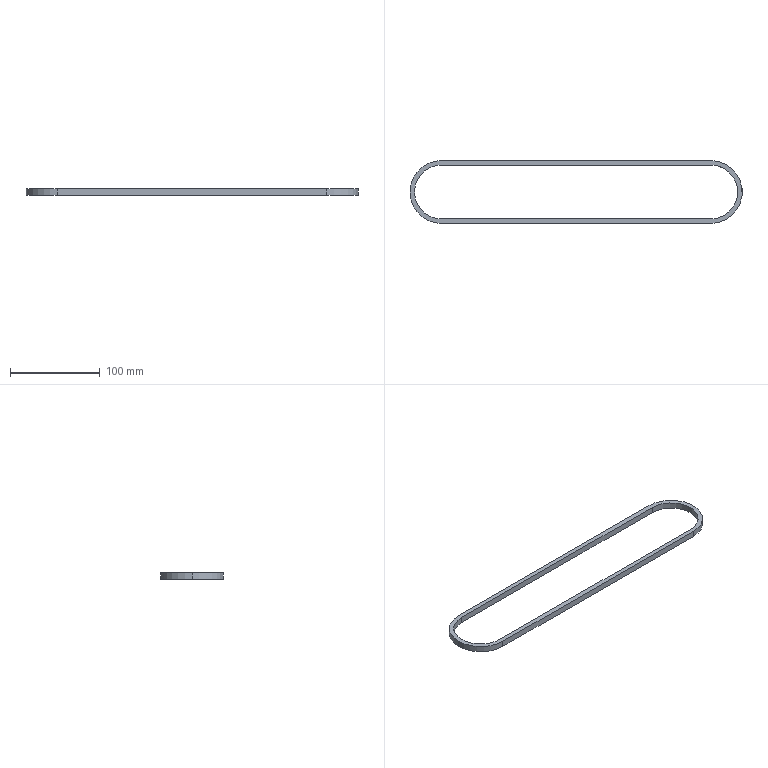Part | SolidWorks | 1 solid | 12 faces | box 370 x 70 x 7 mm | volume 28147 mm3 | cylinder 6 | plane 6 | commonest cylinder face diameters 60 x3 70 x3
STEP:
#1=CARTESIAN_POINT('',(-30.,0.,135.));
#2=VERTEX_POINT('',#1);
#3=CARTESIAN_POINT('',(0.,-30.,135.));
#4=VERTEX_POINT('',#3);
#5=CARTESIAN_POINT('',(0.,0.,135.));
#6=DIRECTION('',(0.,0.,1.));
#7=DIRECTION('',(-1.,0.,0.));
#8=AXIS2_PLACEMENT_3D('',#5,#6,#7);
#9=CIRCLE('',#8,30.);
#10=EDGE_CURVE('',#2,#4,#9,.T.);
#11=ORIENTED_EDGE('',*,*,#10,.T.);
#12=CARTESIAN_POINT('',(0.,-30.,128.));
#13=VERTEX_POINT('',#12);
#14=CARTESIAN_POINT('',(0.,-30.,128.));
#15=DIRECTION('',(0.,0.,1.));
#16=VECTOR('',#15,1000.);
#17=LINE('',#14,#16);
#18=EDGE_CURVE('',#13,#4,#17,.T.);
#19=ORIENTED_EDGE('',*,*,#18,.F.);
#20=CARTESIAN_POINT('',(-30.,0.,128.));
#21=VERTEX_POINT('',#20);
#22=CARTESIAN_POINT('',(0.,0.,128.));
#23=DIRECTION('',(0.,0.,-1.));
#24=DIRECTION('',(0.,-1.,0.));
#25=AXIS2_PLACEMENT_3D('',#22,#23,#24);
#26=CIRCLE('',#25,30.);
#27=EDGE_CURVE('',#13,#21,#26,.T.);
#28=ORIENTED_EDGE('',*,*,#27,.T.);
#29=CARTESIAN_POINT('',(-30.,0.,128.));
#30=DIRECTION('',(0.,0.,1.));
#31=VECTOR('',#30,1000.);
#32=LINE('',#29,#31);
#33=EDGE_CURVE('',#21,#2,#32,.T.);
#34=ORIENTED_EDGE('',*,*,#33,.T.);
#35=EDGE_LOOP('',(#11,#19,#28,#34));
#36=FACE_OUTER_BOUND('',#35,.T.);
#37=CARTESIAN_POINT('',(0.,0.,135.));
#38=DIRECTION('',(0.,0.,-1.));
#39=DIRECTION('',(-1.,0.,0.));
#40=AXIS2_PLACEMENT_3D('',#37,#38,#39);
#41=CYLINDRICAL_SURFACE('',#40,30.);
#42=ADVANCED_FACE('',(#36),#41,.F.);
#43=ORIENTED_EDGE('',*,*,#33,.F.);
#44=CARTESIAN_POINT('',(0.,30.,128.));
#45=VERTEX_POINT('',#44);
#46=CARTESIAN_POINT('',(0.,0.,128.));
#47=DIRECTION('',(0.,0.,-1.));
#48=DIRECTION('',(-1.,0.,0.));
#49=AXIS2_PLACEMENT_3D('',#46,#47,#48);
#50=CIRCLE('',#49,30.);
#51=EDGE_CURVE('',#21,#45,#50,.T.);
#52=ORIENTED_EDGE('',*,*,#51,.T.);
#53=CARTESIAN_POINT('',(0.,30.,135.));
#54=VERTEX_POINT('',#53);
#55=CARTESIAN_POINT('',(0.,30.,135.));
#56=DIRECTION('',(0.,0.,-1.));
#57=VECTOR('',#56,1000.);
#58=LINE('',#55,#57);
#59=EDGE_CURVE('',#54,#45,#58,.T.);
#60=ORIENTED_EDGE('',*,*,#59,.F.);
#61=CARTESIAN_POINT('',(0.,0.,135.));
#62=DIRECTION('',(0.,0.,1.));
#63=DIRECTION('',(0.,1.,0.));
#64=AXIS2_PLACEMENT_3D('',#61,#62,#63);
#65=CIRCLE('',#64,30.);
#66=EDGE_CURVE('',#54,#2,#65,.T.);
#67=ORIENTED_EDGE('',*,*,#66,.T.);
#68=EDGE_LOOP('',(#43,#52,#60,#67));
#69=FACE_OUTER_BOUND('',#68,.T.);
#70=CARTESIAN_POINT('',(0.,0.,135.));
#71=DIRECTION('',(0.,0.,-1.));
#72=DIRECTION('',(-1.,0.,0.));
#73=AXIS2_PLACEMENT_3D('',#70,#71,#72);
#74=CYLINDRICAL_SURFACE('',#73,30.);
#75=ADVANCED_FACE('',(#69),#74,.F.);
#76=CARTESIAN_POINT('',(300.,30.,128.));
#77=VERTEX_POINT('',#76);
#78=CARTESIAN_POINT('',(300.,30.,128.));
#79=DIRECTION('',(-1.,0.,0.));
#80=VECTOR('',#79,1000.);
#81=LINE('',#78,#80);
#82=EDGE_CURVE('',#77,#45,#81,.T.);
#83=ORIENTED_EDGE('',*,*,#82,.F.);
#84=CARTESIAN_POINT('',(300.,30.,135.));
#85=VERTEX_POINT('',#84);
#86=CARTESIAN_POINT('',(300.,30.,128.));
#87=DIRECTION('',(0.,0.,1.));
#88=VECTOR('',#87,1000.);
#89=LINE('',#86,#88);
#90=EDGE_CURVE('',#77,#85,#89,.T.);
#91=ORIENTED_EDGE('',*,*,#90,.T.);
#92=CARTESIAN_POINT('',(300.,30.,135.));
#93=DIRECTION('',(-1.,0.,0.));
#94=VECTOR('',#93,1000.);
#95=LINE('',#92,#94);
#96=EDGE_CURVE('',#85,#54,#95,.T.);
#97=ORIENTED_EDGE('',*,*,#96,.T.);
#98=ORIENTED_EDGE('',*,*,#59,.T.);
#99=EDGE_LOOP('',(#83,#91,#97,#98));
#100=FACE_OUTER_BOUND('',#99,.T.);
#101=CARTESIAN_POINT('',(0.,30.,135.));
#102=DIRECTION('',(0.,1.,0.));
#103=DIRECTION('',(1.,0.,0.));
#104=AXIS2_PLACEMENT_3D('',#101,#102,#103);
#105=PLANE('',#104);
#106=ADVANCED_FACE('',(#100),#105,.F.);
#107=CARTESIAN_POINT('',(300.,-30.,128.));
#108=VERTEX_POINT('',#107);
#109=CARTESIAN_POINT('',(300.,0.,128.));
#110=DIRECTION('',(0.,0.,-1.));
#111=DIRECTION('',(0.,1.,0.));
#112=AXIS2_PLACEMENT_3D('',#109,#110,#111);
#113=CIRCLE('',#112,30.);
#114=EDGE_CURVE('',#77,#108,#113,.T.);
#115=ORIENTED_EDGE('',*,*,#114,.T.);
#116=CARTESIAN_POINT('',(300.,-30.,135.));
#117=VERTEX_POINT('',#116);
#118=CARTESIAN_POINT('',(300.,-30.,135.));
#119=DIRECTION('',(0.,0.,-1.));
#120=VECTOR('',#119,1000.);
#121=LINE('',#118,#120);
#122=EDGE_CURVE('',#117,#108,#121,.T.);
#123=ORIENTED_EDGE('',*,*,#122,.F.);
#124=CARTESIAN_POINT('',(300.,0.,135.));
#125=DIRECTION('',(0.,0.,1.));
#126=DIRECTION('',(0.,-1.,0.));
#127=AXIS2_PLACEMENT_3D('',#124,#125,#126);
#128=CIRCLE('',#127,30.);
#129=EDGE_CURVE('',#117,#85,#128,.T.);
#130=ORIENTED_EDGE('',*,*,#129,.T.);
#131=ORIENTED_EDGE('',*,*,#90,.F.);
#132=EDGE_LOOP('',(#115,#123,#130,#131));
#133=FACE_OUTER_BOUND('',#132,.T.);
#134=CARTESIAN_POINT('',(300.,0.,135.));
#135=DIRECTION('',(0.,0.,-1.));
#136=DIRECTION('',(-1.,0.,0.));
#137=AXIS2_PLACEMENT_3D('',#134,#135,#136);
#138=CYLINDRICAL_SURFACE('',#137,30.);
#139=ADVANCED_FACE('',(#133),#138,.F.);
#140=CARTESIAN_POINT('',(0.,-30.,128.));
#141=DIRECTION('',(1.,0.,0.));
#142=VECTOR('',#141,1000.);
#143=LINE('',#140,#142);
#144=EDGE_CURVE('',#13,#108,#143,.T.);
#145=ORIENTED_EDGE('',*,*,#144,.F.);
#146=ORIENTED_EDGE('',*,*,#18,.T.);
#147=CARTESIAN_POINT('',(0.,-30.,135.));
#148=DIRECTION('',(1.,0.,0.));
#149=VECTOR('',#148,1000.);
#150=LINE('',#147,#149);
#151=EDGE_CURVE('',#4,#117,#150,.T.);
#152=ORIENTED_EDGE('',*,*,#151,.T.);
#153=ORIENTED_EDGE('',*,*,#122,.T.);
#154=EDGE_LOOP('',(#145,#146,#152,#153));
#155=FACE_OUTER_BOUND('',#154,.T.);
#156=CARTESIAN_POINT('',(300.,-30.,135.));
#157=DIRECTION('',(0.,-1.,0.));
#158=DIRECTION('',(0.,0.,-1.));
#159=AXIS2_PLACEMENT_3D('',#156,#157,#158);
#160=PLANE('',#159);
#161=ADVANCED_FACE('',(#155),#160,.F.);
#162=CARTESIAN_POINT('',(300.,35.,128.));
#163=VERTEX_POINT('',#162);
#164=CARTESIAN_POINT('',(0.,35.,128.));
#165=VERTEX_POINT('',#164);
#166=CARTESIAN_POINT('',(300.,35.,128.));
#167=DIRECTION('',(-1.,0.,0.));
#168=VECTOR('',#167,1000.);
#169=LINE('',#166,#168);
#170=EDGE_CURVE('',#163,#165,#169,.T.);
#171=ORIENTED_EDGE('',*,*,#170,.T.);
#172=CARTESIAN_POINT('',(0.,35.,135.));
#173=VERTEX_POINT('',#172);
#174=CARTESIAN_POINT('',(0.,35.,128.));
#175=DIRECTION('',(0.,0.,1.));
#176=VECTOR('',#175,1000.);
#177=LINE('',#174,#176);
#178=EDGE_CURVE('',#165,#173,#177,.T.);
#179=ORIENTED_EDGE('',*,*,#178,.T.);
#180=CARTESIAN_POINT('',(300.,35.,135.));
#181=VERTEX_POINT('',#180);
#182=CARTESIAN_POINT('',(300.,35.,135.));
#183=DIRECTION('',(-1.,0.,0.));
#184=VECTOR('',#183,1000.);
#185=LINE('',#182,#184);
#186=EDGE_CURVE('',#181,#173,#185,.T.);
#187=ORIENTED_EDGE('',*,*,#186,.F.);
#188=CARTESIAN_POINT('',(300.,35.,135.));
#189=DIRECTION('',(0.,0.,-1.));
#190=VECTOR('',#189,1000.);
#191=LINE('',#188,#190);
#192=EDGE_CURVE('',#181,#163,#191,.T.);
#193=ORIENTED_EDGE('',*,*,#192,.T.);
#194=EDGE_LOOP('',(#171,#179,#187,#193));
#195=FACE_OUTER_BOUND('',#194,.T.);
#196=CARTESIAN_POINT('',(0.,35.,135.));
#197=DIRECTION('',(0.,1.,0.));
#198=DIRECTION('',(1.,0.,0.));
#199=AXIS2_PLACEMENT_3D('',#196,#197,#198);
#200=PLANE('',#199);
#201=ADVANCED_FACE('',(#195),#200,.T.);
#202=ORIENTED_EDGE('',*,*,#144,.T.);
#203=ORIENTED_EDGE('',*,*,#114,.F.);
#204=ORIENTED_EDGE('',*,*,#82,.T.);
#205=ORIENTED_EDGE('',*,*,#51,.F.);
#206=ORIENTED_EDGE('',*,*,#27,.F.);
#207=EDGE_LOOP('',(#202,#203,#204,#205,#206));
#208=FACE_BOUND('',#207,.T.);
#209=CARTESIAN_POINT('',(-35.,0.,128.));
#210=VERTEX_POINT('',#209);
#211=CARTESIAN_POINT('',(0.,-35.,128.));
#212=VERTEX_POINT('',#211);
#213=CARTESIAN_POINT('',(0.,0.,128.));
#214=DIRECTION('',(0.,0.,1.));
#215=DIRECTION('',(-1.,0.,0.));
#216=AXIS2_PLACEMENT_3D('',#213,#214,#215);
#217=CIRCLE('',#216,35.);
#218=EDGE_CURVE('',#210,#212,#217,.T.);
#219=ORIENTED_EDGE('',*,*,#218,.F.);
#220=CARTESIAN_POINT('',(0.,0.,128.));
#221=DIRECTION('',(0.,0.,1.));
#222=DIRECTION('',(0.,1.,0.));
#223=AXIS2_PLACEMENT_3D('',#220,#221,#222);
#224=CIRCLE('',#223,35.);
#225=EDGE_CURVE('',#165,#210,#224,.T.);
#226=ORIENTED_EDGE('',*,*,#225,.F.);
#227=ORIENTED_EDGE('',*,*,#170,.F.);
#228=CARTESIAN_POINT('',(300.,-35.,128.));
#229=VERTEX_POINT('',#228);
#230=CARTESIAN_POINT('',(300.,0.,128.));
#231=DIRECTION('',(0.,0.,1.));
#232=DIRECTION('',(1.,0.,0.));
#233=AXIS2_PLACEMENT_3D('',#230,#231,#232);
#234=CIRCLE('',#233,35.);
#235=EDGE_CURVE('',#229,#163,#234,.T.);
#236=ORIENTED_EDGE('',*,*,#235,.F.);
#237=CARTESIAN_POINT('',(0.,-35.,128.));
#238=DIRECTION('',(1.,0.,0.));
#239=VECTOR('',#238,1000.);
#240=LINE('',#237,#239);
#241=EDGE_CURVE('',#212,#229,#240,.T.);
#242=ORIENTED_EDGE('',*,*,#241,.F.);
#243=EDGE_LOOP('',(#219,#226,#227,#236,#242));
#244=FACE_OUTER_BOUND('',#243,.T.);
#245=CARTESIAN_POINT('',(150.,32.5,128.));
#246=DIRECTION('',(0.,0.,-1.));
#247=DIRECTION('',(0.,-1.,0.));
#248=AXIS2_PLACEMENT_3D('',#245,#246,#247);
#249=PLANE('',#248);
#250=ADVANCED_FACE('',(#208,#244),#249,.T.);
#251=CARTESIAN_POINT('',(-35.,0.,135.));
#252=VERTEX_POINT('',#251);
#253=CARTESIAN_POINT('',(0.,0.,135.));
#254=DIRECTION('',(0.,0.,-1.));
#255=DIRECTION('',(-1.,0.,0.));
#256=AXIS2_PLACEMENT_3D('',#253,#254,#255);
#257=CIRCLE('',#256,35.);
#258=EDGE_CURVE('',#252,#173,#257,.T.);
#259=ORIENTED_EDGE('',*,*,#258,.T.);
#260=ORIENTED_EDGE('',*,*,#178,.F.);
#261=ORIENTED_EDGE('',*,*,#225,.T.);
#262=CARTESIAN_POINT('',(-35.,0.,128.));
#263=DIRECTION('',(0.,0.,1.));
#264=VECTOR('',#263,1000.);
#265=LINE('',#262,#264);
#266=EDGE_CURVE('',#210,#252,#265,.T.);
#267=ORIENTED_EDGE('',*,*,#266,.T.);
#268=EDGE_LOOP('',(#259,#260,#261,#267));
#269=FACE_OUTER_BOUND('',#268,.T.);
#270=CARTESIAN_POINT('',(0.,0.,135.));
#271=DIRECTION('',(0.,0.,-1.));
#272=DIRECTION('',(-1.,0.,0.));
#273=AXIS2_PLACEMENT_3D('',#270,#271,#272);
#274=CYLINDRICAL_SURFACE('',#273,35.);
#275=ADVANCED_FACE('',(#269),#274,.T.);
#276=ORIENTED_EDGE('',*,*,#10,.F.);
#277=ORIENTED_EDGE('',*,*,#66,.F.);
#278=ORIENTED_EDGE('',*,*,#96,.F.);
#279=ORIENTED_EDGE('',*,*,#129,.F.);
#280=ORIENTED_EDGE('',*,*,#151,.F.);
#281=EDGE_LOOP('',(#276,#277,#278,#279,#280));
#282=FACE_BOUND('',#281,.T.);
#283=CARTESIAN_POINT('',(300.,-35.,135.));
#284=VERTEX_POINT('',#283);
#285=CARTESIAN_POINT('',(300.,0.,135.));
#286=DIRECTION('',(0.,0.,-1.));
#287=DIRECTION('',(1.,0.,0.));
#288=AXIS2_PLACEMENT_3D('',#285,#286,#287);
#289=CIRCLE('',#288,35.);
#290=EDGE_CURVE('',#181,#284,#289,.T.);
#291=ORIENTED_EDGE('',*,*,#290,.F.);
#292=ORIENTED_EDGE('',*,*,#186,.T.);
#293=ORIENTED_EDGE('',*,*,#258,.F.);
#294=CARTESIAN_POINT('',(0.,-35.,135.));
#295=VERTEX_POINT('',#294);
#296=CARTESIAN_POINT('',(0.,0.,135.));
#297=DIRECTION('',(0.,0.,-1.));
#298=DIRECTION('',(0.,-1.,0.));
#299=AXIS2_PLACEMENT_3D('',#296,#297,#298);
#300=CIRCLE('',#299,35.);
#301=EDGE_CURVE('',#295,#252,#300,.T.);
#302=ORIENTED_EDGE('',*,*,#301,.F.);
#303=CARTESIAN_POINT('',(0.,-35.,135.));
#304=DIRECTION('',(1.,0.,0.));
#305=VECTOR('',#304,1000.);
#306=LINE('',#303,#305);
#307=EDGE_CURVE('',#295,#284,#306,.T.);
#308=ORIENTED_EDGE('',*,*,#307,.T.);
#309=EDGE_LOOP('',(#291,#292,#293,#302,#308));
#310=FACE_OUTER_BOUND('',#309,.T.);
#311=CARTESIAN_POINT('',(150.,32.5,135.));
#312=DIRECTION('',(0.,0.,-1.));
#313=DIRECTION('',(0.,-1.,0.));
#314=AXIS2_PLACEMENT_3D('',#311,#312,#313);
#315=PLANE('',#314);
#316=ADVANCED_FACE('',(#282,#310),#315,.F.);
#317=ORIENTED_EDGE('',*,*,#266,.F.);
#318=ORIENTED_EDGE('',*,*,#218,.T.);
#319=CARTESIAN_POINT('',(0.,-35.,135.));
#320=DIRECTION('',(0.,0.,-1.));
#321=VECTOR('',#320,1000.);
#322=LINE('',#319,#321);
#323=EDGE_CURVE('',#295,#212,#322,.T.);
#324=ORIENTED_EDGE('',*,*,#323,.F.);
#325=ORIENTED_EDGE('',*,*,#301,.T.);
#326=EDGE_LOOP('',(#317,#318,#324,#325));
#327=FACE_OUTER_BOUND('',#326,.T.);
#328=CARTESIAN_POINT('',(0.,0.,135.));
#329=DIRECTION('',(0.,0.,-1.));
#330=DIRECTION('',(-1.,0.,0.));
#331=AXIS2_PLACEMENT_3D('',#328,#329,#330);
#332=CYLINDRICAL_SURFACE('',#331,35.);
#333=ADVANCED_FACE('',(#327),#332,.T.);
#334=ORIENTED_EDGE('',*,*,#241,.T.);
#335=CARTESIAN_POINT('',(300.,-35.,128.));
#336=DIRECTION('',(0.,0.,1.));
#337=VECTOR('',#336,1000.);
#338=LINE('',#335,#337);
#339=EDGE_CURVE('',#229,#284,#338,.T.);
#340=ORIENTED_EDGE('',*,*,#339,.T.);
#341=ORIENTED_EDGE('',*,*,#307,.F.);
#342=ORIENTED_EDGE('',*,*,#323,.T.);
#343=EDGE_LOOP('',(#334,#340,#341,#342));
#344=FACE_OUTER_BOUND('',#343,.T.);
#345=CARTESIAN_POINT('',(300.,-35.,135.));
#346=DIRECTION('',(0.,-1.,0.));
#347=DIRECTION('',(0.,0.,-1.));
#348=AXIS2_PLACEMENT_3D('',#345,#346,#347);
#349=PLANE('',#348);
#350=ADVANCED_FACE('',(#344),#349,.T.);
#351=ORIENTED_EDGE('',*,*,#339,.F.);
#352=ORIENTED_EDGE('',*,*,#235,.T.);
#353=ORIENTED_EDGE('',*,*,#192,.F.);
#354=ORIENTED_EDGE('',*,*,#290,.T.);
#355=EDGE_LOOP('',(#351,#352,#353,#354));
#356=FACE_OUTER_BOUND('',#355,.T.);
#357=CARTESIAN_POINT('',(300.,0.,135.));
#358=DIRECTION('',(0.,0.,-1.));
#359=DIRECTION('',(-1.,0.,0.));
#360=AXIS2_PLACEMENT_3D('',#357,#358,#359);
#361=CYLINDRICAL_SURFACE('',#360,35.);
#362=ADVANCED_FACE('',(#356),#361,.T.);
#363=CLOSED_SHELL('',(#42,#75,#106,#139,#161,#201,#250,#275,#316,#333,#350,#362));
#364=MANIFOLD_SOLID_BREP('',#363);
#365=CARTESIAN_POINT('',(0.,0.,0.));
#366=DIRECTION('',(0.,0.,1.));
#367=DIRECTION('',(1.,0.,0.));
#368=AXIS2_PLACEMENT_3D('',#365,#366,#367);
#369=(LENGTH_UNIT()NAMED_UNIT(*)SI_UNIT(.MILLI.,.METRE.));
#370=UNCERTAINTY_MEASURE_WITH_UNIT(LENGTH_MEASURE(0.00001),#369,'','');
#371=(NAMED_UNIT(*)PLANE_ANGLE_UNIT()SI_UNIT($,.RADIAN.));
#372=(NAMED_UNIT(*)SI_UNIT($,.STERADIAN.)SOLID_ANGLE_UNIT());
#373=(GEOMETRIC_REPRESENTATION_CONTEXT(3)GLOBAL_UNCERTAINTY_ASSIGNED_CONTEXT((#370))GLOBAL_UNIT_ASSIGNED_CONTEXT((#369,#371,#372))REPRESENTATION_CONTEXT('',''));
#374=ADVANCED_BREP_SHAPE_REPRESENTATION('',(#364,#368),#373);